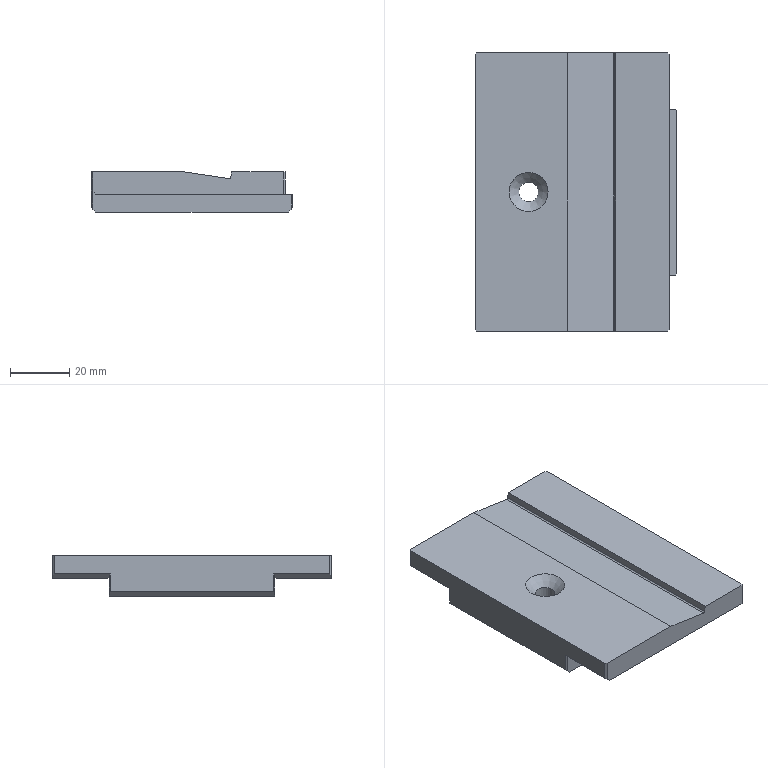NC program | NX | posted with a generic post | part box 68 x 94 x 13.65 mm
Whole program:
N10 G17 G21 G94 G90
(FLOOR_FACING , TOOL : D12开粗)
N12 T02 M6
N14 G54
N16 G17 G0 G90 X56.1 Y-13.303 B0. C0. S6500 M3
N18 G43 Z30. H2
N20 Z3.1
N22 G94 G1 Z0.1 F1000.
N24 X53.1
N26 X-53.1
N28 Y-6.3
N30 X53.1
N32 X56.1
N34 Z3.1
N36 G0 Z30.
N38 M5
(PLANAR_MILL_2 , TOOL : D4R0.5)
N40 T07 M6
N42 G54
N44 G17 G0 G90 X50.998 Y-2.098 B0. C0. S6500 M3
N46 G43 Z30. H7
N48 Z4.94
N50 G94 G1 Z1.94 F1000.
N52 X47.
N54 X-47.
N56 X-50.998
N58 Z4.94
N60 G0 Z30.
N62 X51. Y-2.1
N64 Z4.48
N66 G1 Z1.48
N68 X47.
N70 X-47.
N72 X-51.
N74 Z4.48
N76 G0 Z30.
N78 X51.
N80 Z4.02
N82 G1 Z1.02
N84 X47.
N86 X-47.
N88 X-51.
N90 Z4.02
N92 G0 Z30.
N94 X51.
N96 Z3.56
N98 G1 Z0.56
N100 X47.
N102 X-47.
N104 X-51.
N106 Z3.56
N108 G0 Z30.
N110 X51.
N112 Z3.1
N114 G1 Z0.1
N116 X47.
N118 X-47.
N120 X-51.
N122 Z3.1
N124 G0 Z30.
(PLANAR_MILL_2_COPY , TOOL : D4R0.5)
N126 X51. Y-2.
N128 Z3.
N130 G1 Z0. F800.
N132 X47.
N134 X-47.
N136 X-51.
N138 Z3.
N140 G0 Z30.
(FLOOR_FACING_COPY , TOOL : D4R0.5)
N142 X52. Y-16.2
N144 Z3.
N146 G1 Z0. F1000.
N148 X49.
N150 X-49.
N152 Y-14.243
N154 X49.
N156 Y-12.286
N158 X-49.
N160 Y-10.329
N162 X49.
N164 Y-8.372
N166 X-49.
N168 Y-6.414
N170 X49.
N172 Y-4.457
N174 X-49.
N176 Y-2.5
N178 X49.
N180 X52.
N182 Z3.
N184 G0 Z30.
N186 M5
N188 M2